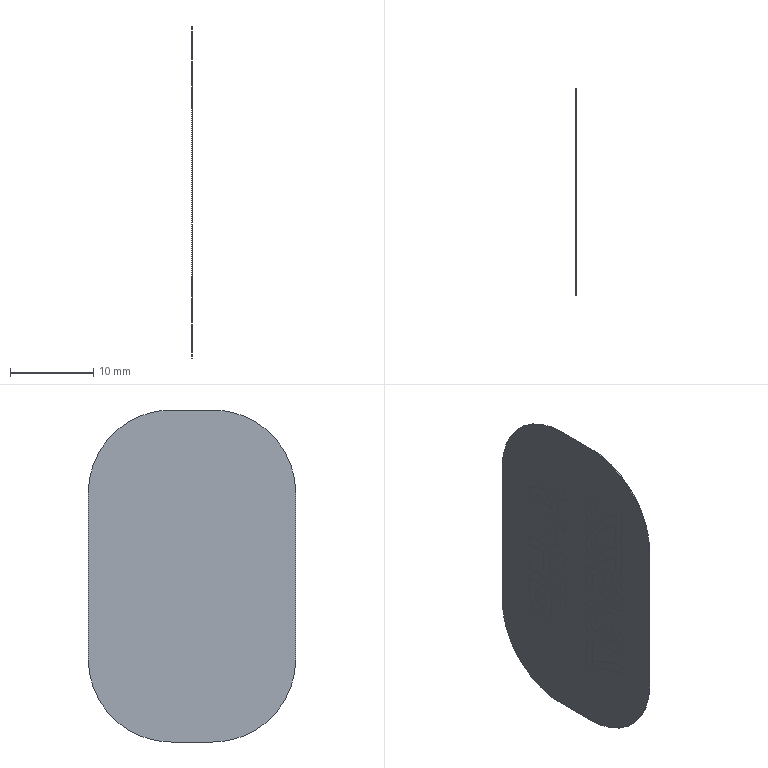Part | STEP file | a-hp_225_37-140_3_0_03 | 1 solid | 134 faces | box 0.1 x 25 x 40 mm | volume 85.323 mm3 | plane 80 | spline 50 | cylinder 4 | commonest cylinder face diameters 20 x4